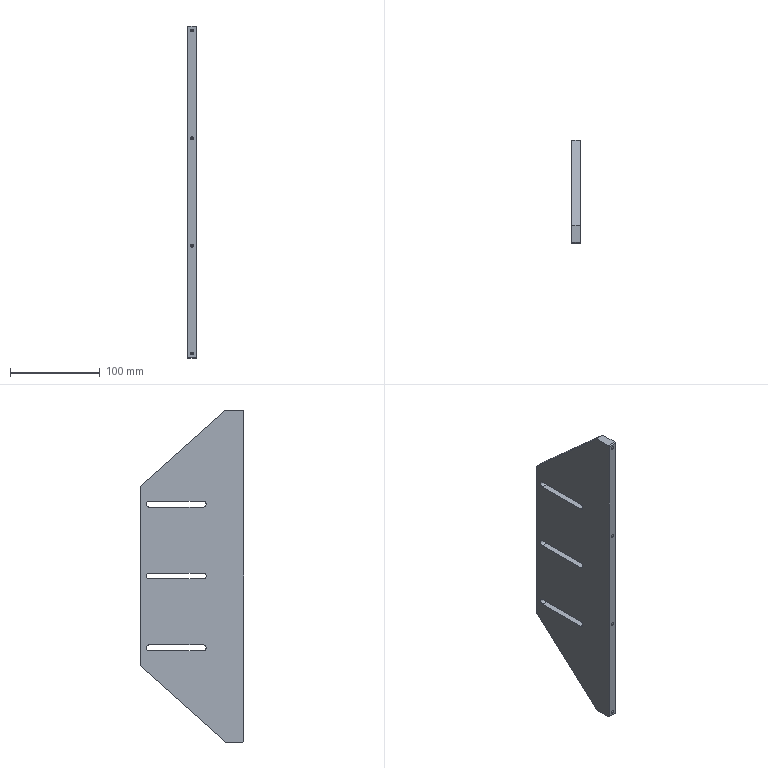Part | SolidWorks | features HoleWzd 2, Chamfer 1, Extrusion 1, ICE 1 | 1 solid | 38 faces | box 10 x 115 x 370 mm | volume 331477 mm3 | plane 16 | cylinder 14 | cone 8 | commonest cylinder face diameters 3.3 x8 6.6 x6
STEP:
#1=CARTESIAN_POINT('',(0.,-104.9,181.65));
#2=VERTEX_POINT('',#1);
#3=CARTESIAN_POINT('',(0.,-104.9,178.35));
#4=VERTEX_POINT('',#3);
#5=CARTESIAN_POINT('',(0.,-104.9,180.));
#6=DIRECTION('',(0.,-1.,0.));
#7=DIRECTION('',(0.,0.,-1.));
#8=AXIS2_PLACEMENT_3D('',#5,#6,#7);
#9=CIRCLE('',#8,1.65);
#10=EDGE_CURVE('',#2,#4,#9,.T.);
#11=ORIENTED_EDGE('',*,*,#10,.F.);
#12=CARTESIAN_POINT('',(0.,-115.,181.65));
#13=VERTEX_POINT('',#12);
#14=CARTESIAN_POINT('',(0.,-115.,181.65));
#15=DIRECTION('',(0.,-1.,0.));
#16=VECTOR('',#15,1000.);
#17=LINE('',#14,#16);
#18=EDGE_CURVE('',#2,#13,#17,.T.);
#19=ORIENTED_EDGE('',*,*,#18,.T.);
#20=CARTESIAN_POINT('',(0.,-115.,178.35));
#21=VERTEX_POINT('',#20);
#22=CARTESIAN_POINT('',(0.,-115.,180.));
#23=DIRECTION('',(0.,-1.,0.));
#24=DIRECTION('',(0.,0.,-1.));
#25=AXIS2_PLACEMENT_3D('',#22,#23,#24);
#26=CIRCLE('',#25,1.65);
#27=EDGE_CURVE('',#13,#21,#26,.T.);
#28=ORIENTED_EDGE('',*,*,#27,.T.);
#29=CARTESIAN_POINT('',(0.,-115.,178.35));
#30=DIRECTION('',(0.,-1.,0.));
#31=VECTOR('',#30,1000.);
#32=LINE('',#29,#31);
#33=EDGE_CURVE('',#4,#21,#32,.T.);
#34=ORIENTED_EDGE('',*,*,#33,.F.);
#35=EDGE_LOOP('',(#11,#19,#28,#34));
#36=FACE_OUTER_BOUND('',#35,.T.);
#37=CARTESIAN_POINT('',(0.,-115.,180.));
#38=DIRECTION('',(0.,-1.,0.));
#39=DIRECTION('',(0.,0.,-1.));
#40=AXIS2_PLACEMENT_3D('',#37,#38,#39);
#41=CYLINDRICAL_SURFACE('',#40,1.65);
#42=ADVANCED_FACE('',(#36),#41,.F.);
#43=CARTESIAN_POINT('',(0.,-103.909,180.));
#44=VERTEX_POINT('',#43);
#45=CARTESIAN_POINT('',(0.,-104.9,178.35));
#46=DIRECTION('',(0.,-0.515,-0.8572));
#47=VECTOR('',#46,1000.);
#48=LINE('',#45,#47);
#49=EDGE_CURVE('',#44,#4,#48,.T.);
#50=ORIENTED_EDGE('',*,*,#49,.F.);
#51=CARTESIAN_POINT('',(0.,-104.9,181.65));
#52=DIRECTION('',(0.,-0.515,0.8572));
#53=VECTOR('',#52,1000.);
#54=LINE('',#51,#53);
#55=EDGE_CURVE('',#44,#2,#54,.T.);
#56=ORIENTED_EDGE('',*,*,#55,.T.);
#57=ORIENTED_EDGE('',*,*,#10,.T.);
#58=EDGE_LOOP('',(#50,#56,#57));
#59=FACE_OUTER_BOUND('',#58,.T.);
#60=CARTESIAN_POINT('',(0.,-104.9,180.));
#61=DIRECTION('',(0.,-1.,0.));
#62=DIRECTION('',(0.,0.,-1.));
#63=AXIS2_PLACEMENT_3D('',#60,#61,#62);
#64=CONICAL_SURFACE('',#63,1.65,1.03);
#65=ADVANCED_FACE('',(#59),#64,.F.);
#66=CARTESIAN_POINT('',(0.,-104.9,61.65));
#67=VERTEX_POINT('',#66);
#68=CARTESIAN_POINT('',(0.,-104.9,58.35));
#69=VERTEX_POINT('',#68);
#70=CARTESIAN_POINT('',(0.,-104.9,60.));
#71=DIRECTION('',(0.,-1.,0.));
#72=DIRECTION('',(0.,0.,-1.));
#73=AXIS2_PLACEMENT_3D('',#70,#71,#72);
#74=CIRCLE('',#73,1.65);
#75=EDGE_CURVE('',#67,#69,#74,.T.);
#76=ORIENTED_EDGE('',*,*,#75,.F.);
#77=CARTESIAN_POINT('',(0.,-115.,61.65));
#78=VERTEX_POINT('',#77);
#79=CARTESIAN_POINT('',(0.,-115.,61.65));
#80=DIRECTION('',(0.,-1.,0.));
#81=VECTOR('',#80,1000.);
#82=LINE('',#79,#81);
#83=EDGE_CURVE('',#67,#78,#82,.T.);
#84=ORIENTED_EDGE('',*,*,#83,.T.);
#85=CARTESIAN_POINT('',(0.,-115.,58.35));
#86=VERTEX_POINT('',#85);
#87=CARTESIAN_POINT('',(0.,-115.,60.));
#88=DIRECTION('',(0.,-1.,0.));
#89=DIRECTION('',(0.,0.,-1.));
#90=AXIS2_PLACEMENT_3D('',#87,#88,#89);
#91=CIRCLE('',#90,1.65);
#92=EDGE_CURVE('',#78,#86,#91,.T.);
#93=ORIENTED_EDGE('',*,*,#92,.T.);
#94=CARTESIAN_POINT('',(0.,-115.,58.35));
#95=DIRECTION('',(0.,-1.,0.));
#96=VECTOR('',#95,1000.);
#97=LINE('',#94,#96);
#98=EDGE_CURVE('',#69,#86,#97,.T.);
#99=ORIENTED_EDGE('',*,*,#98,.F.);
#100=EDGE_LOOP('',(#76,#84,#93,#99));
#101=FACE_OUTER_BOUND('',#100,.T.);
#102=CARTESIAN_POINT('',(0.,-115.,60.));
#103=DIRECTION('',(0.,-1.,0.));
#104=DIRECTION('',(0.,0.,-1.));
#105=AXIS2_PLACEMENT_3D('',#102,#103,#104);
#106=CYLINDRICAL_SURFACE('',#105,1.65);
#107=ADVANCED_FACE('',(#101),#106,.F.);
#108=CARTESIAN_POINT('',(0.,-103.909,60.));
#109=VERTEX_POINT('',#108);
#110=CARTESIAN_POINT('',(0.,-104.9,58.35));
#111=DIRECTION('',(0.,-0.515,-0.8572));
#112=VECTOR('',#111,1000.);
#113=LINE('',#110,#112);
#114=EDGE_CURVE('',#109,#69,#113,.T.);
#115=ORIENTED_EDGE('',*,*,#114,.F.);
#116=CARTESIAN_POINT('',(0.,-104.9,61.65));
#117=DIRECTION('',(0.,-0.515,0.8572));
#118=VECTOR('',#117,1000.);
#119=LINE('',#116,#118);
#120=EDGE_CURVE('',#109,#67,#119,.T.);
#121=ORIENTED_EDGE('',*,*,#120,.T.);
#122=ORIENTED_EDGE('',*,*,#75,.T.);
#123=EDGE_LOOP('',(#115,#121,#122));
#124=FACE_OUTER_BOUND('',#123,.T.);
#125=CARTESIAN_POINT('',(0.,-104.9,60.));
#126=DIRECTION('',(0.,-1.,0.));
#127=DIRECTION('',(0.,0.,-1.));
#128=AXIS2_PLACEMENT_3D('',#125,#126,#127);
#129=CONICAL_SURFACE('',#128,1.65,1.03);
#130=ADVANCED_FACE('',(#124),#129,.F.);
#131=CARTESIAN_POINT('',(0.,-104.9,-58.35));
#132=VERTEX_POINT('',#131);
#133=CARTESIAN_POINT('',(0.,-104.9,-61.65));
#134=VERTEX_POINT('',#133);
#135=CARTESIAN_POINT('',(0.,-104.9,-60.));
#136=DIRECTION('',(0.,-1.,0.));
#137=DIRECTION('',(0.,0.,-1.));
#138=AXIS2_PLACEMENT_3D('',#135,#136,#137);
#139=CIRCLE('',#138,1.65);
#140=EDGE_CURVE('',#132,#134,#139,.T.);
#141=ORIENTED_EDGE('',*,*,#140,.F.);
#142=CARTESIAN_POINT('',(0.,-115.,-58.35));
#143=VERTEX_POINT('',#142);
#144=CARTESIAN_POINT('',(0.,-115.,-58.35));
#145=DIRECTION('',(0.,-1.,0.));
#146=VECTOR('',#145,1000.);
#147=LINE('',#144,#146);
#148=EDGE_CURVE('',#132,#143,#147,.T.);
#149=ORIENTED_EDGE('',*,*,#148,.T.);
#150=CARTESIAN_POINT('',(0.,-115.,-61.65));
#151=VERTEX_POINT('',#150);
#152=CARTESIAN_POINT('',(0.,-115.,-60.));
#153=DIRECTION('',(0.,-1.,0.));
#154=DIRECTION('',(0.,0.,-1.));
#155=AXIS2_PLACEMENT_3D('',#152,#153,#154);
#156=CIRCLE('',#155,1.65);
#157=EDGE_CURVE('',#143,#151,#156,.T.);
#158=ORIENTED_EDGE('',*,*,#157,.T.);
#159=CARTESIAN_POINT('',(0.,-115.,-61.65));
#160=DIRECTION('',(0.,-1.,0.));
#161=VECTOR('',#160,1000.);
#162=LINE('',#159,#161);
#163=EDGE_CURVE('',#134,#151,#162,.T.);
#164=ORIENTED_EDGE('',*,*,#163,.F.);
#165=EDGE_LOOP('',(#141,#149,#158,#164));
#166=FACE_OUTER_BOUND('',#165,.T.);
#167=CARTESIAN_POINT('',(0.,-115.,-60.));
#168=DIRECTION('',(0.,-1.,0.));
#169=DIRECTION('',(0.,0.,-1.));
#170=AXIS2_PLACEMENT_3D('',#167,#168,#169);
#171=CYLINDRICAL_SURFACE('',#170,1.65);
#172=ADVANCED_FACE('',(#166),#171,.F.);
#173=CARTESIAN_POINT('',(0.,-103.909,-60.));
#174=VERTEX_POINT('',#173);
#175=CARTESIAN_POINT('',(0.,-104.9,-61.65));
#176=DIRECTION('',(0.,-0.515,-0.8572));
#177=VECTOR('',#176,1000.);
#178=LINE('',#175,#177);
#179=EDGE_CURVE('',#174,#134,#178,.T.);
#180=ORIENTED_EDGE('',*,*,#179,.F.);
#181=CARTESIAN_POINT('',(0.,-104.9,-58.35));
#182=DIRECTION('',(0.,-0.515,0.8572));
#183=VECTOR('',#182,1000.);
#184=LINE('',#181,#183);
#185=EDGE_CURVE('',#174,#132,#184,.T.);
#186=ORIENTED_EDGE('',*,*,#185,.T.);
#187=ORIENTED_EDGE('',*,*,#140,.T.);
#188=EDGE_LOOP('',(#180,#186,#187));
#189=FACE_OUTER_BOUND('',#188,.T.);
#190=CARTESIAN_POINT('',(0.,-104.9,-60.));
#191=DIRECTION('',(0.,-1.,0.));
#192=DIRECTION('',(0.,0.,-1.));
#193=AXIS2_PLACEMENT_3D('',#190,#191,#192);
#194=CONICAL_SURFACE('',#193,1.65,1.03);
#195=ADVANCED_FACE('',(#189),#194,.F.);
#196=CARTESIAN_POINT('',(0.,-104.9,-178.35));
#197=VERTEX_POINT('',#196);
#198=CARTESIAN_POINT('',(0.,-104.9,-181.65));
#199=VERTEX_POINT('',#198);
#200=CARTESIAN_POINT('',(0.,-104.9,-180.));
#201=DIRECTION('',(0.,-1.,0.));
#202=DIRECTION('',(0.,0.,-1.));
#203=AXIS2_PLACEMENT_3D('',#200,#201,#202);
#204=CIRCLE('',#203,1.65);
#205=EDGE_CURVE('',#197,#199,#204,.T.);
#206=ORIENTED_EDGE('',*,*,#205,.F.);
#207=CARTESIAN_POINT('',(0.,-115.,-178.35));
#208=VERTEX_POINT('',#207);
#209=CARTESIAN_POINT('',(0.,-115.,-178.35));
#210=DIRECTION('',(0.,-1.,0.));
#211=VECTOR('',#210,1000.);
#212=LINE('',#209,#211);
#213=EDGE_CURVE('',#197,#208,#212,.T.);
#214=ORIENTED_EDGE('',*,*,#213,.T.);
#215=CARTESIAN_POINT('',(0.,-115.,-181.65));
#216=VERTEX_POINT('',#215);
#217=CARTESIAN_POINT('',(0.,-115.,-180.));
#218=DIRECTION('',(0.,-1.,0.));
#219=DIRECTION('',(0.,0.,-1.));
#220=AXIS2_PLACEMENT_3D('',#217,#218,#219);
#221=CIRCLE('',#220,1.65);
#222=EDGE_CURVE('',#208,#216,#221,.T.);
#223=ORIENTED_EDGE('',*,*,#222,.T.);
#224=CARTESIAN_POINT('',(0.,-115.,-181.65));
#225=DIRECTION('',(0.,-1.,0.));
#226=VECTOR('',#225,1000.);
#227=LINE('',#224,#226);
#228=EDGE_CURVE('',#199,#216,#227,.T.);
#229=ORIENTED_EDGE('',*,*,#228,.F.);
#230=EDGE_LOOP('',(#206,#214,#223,#229));
#231=FACE_OUTER_BOUND('',#230,.T.);
#232=CARTESIAN_POINT('',(0.,-115.,-180.));
#233=DIRECTION('',(0.,-1.,0.));
#234=DIRECTION('',(0.,0.,-1.));
#235=AXIS2_PLACEMENT_3D('',#232,#233,#234);
#236=CYLINDRICAL_SURFACE('',#235,1.65);
#237=ADVANCED_FACE('',(#231),#236,.F.);
#238=CARTESIAN_POINT('',(0.,-103.909,-180.));
#239=VERTEX_POINT('',#238);
#240=CARTESIAN_POINT('',(0.,-104.9,-181.65));
#241=DIRECTION('',(0.,-0.515,-0.8572));
#242=VECTOR('',#241,1000.);
#243=LINE('',#240,#242);
#244=EDGE_CURVE('',#239,#199,#243,.T.);
#245=ORIENTED_EDGE('',*,*,#244,.F.);
#246=CARTESIAN_POINT('',(0.,-104.9,-178.35));
#247=DIRECTION('',(0.,-0.515,0.8572));
#248=VECTOR('',#247,1000.);
#249=LINE('',#246,#248);
#250=EDGE_CURVE('',#239,#197,#249,.T.);
#251=ORIENTED_EDGE('',*,*,#250,.T.);
#252=ORIENTED_EDGE('',*,*,#205,.T.);
#253=EDGE_LOOP('',(#245,#251,#252));
#254=FACE_OUTER_BOUND('',#253,.T.);
#255=CARTESIAN_POINT('',(0.,-104.9,-180.));
#256=DIRECTION('',(0.,-1.,0.));
#257=DIRECTION('',(0.,0.,-1.));
#258=AXIS2_PLACEMENT_3D('',#255,#256,#257);
#259=CONICAL_SURFACE('',#258,1.65,1.03);
#260=ADVANCED_FACE('',(#254),#259,.F.);
#261=CARTESIAN_POINT('',(-5.,-70.,83.3));
#262=VERTEX_POINT('',#261);
#263=CARTESIAN_POINT('',(-5.,-70.,76.7));
#264=VERTEX_POINT('',#263);
#265=CARTESIAN_POINT('',(-5.,-70.,80.));
#266=DIRECTION('',(1.,0.,0.));
#267=DIRECTION('',(0.,0.,-1.));
#268=AXIS2_PLACEMENT_3D('',#265,#266,#267);
#269=CIRCLE('',#268,3.3);
#270=EDGE_CURVE('',#262,#264,#269,.T.);
#271=ORIENTED_EDGE('',*,*,#270,.T.);
#272=CARTESIAN_POINT('',(-5.,-10.,76.7));
#273=VERTEX_POINT('',#272);
#274=CARTESIAN_POINT('',(-5.,-70.,76.7));
#275=DIRECTION('',(0.,1.,0.));
#276=VECTOR('',#275,1000.);
#277=LINE('',#274,#276);
#278=EDGE_CURVE('',#264,#273,#277,.T.);
#279=ORIENTED_EDGE('',*,*,#278,.T.);
#280=CARTESIAN_POINT('',(-5.,-10.,83.3));
#281=VERTEX_POINT('',#280);
#282=CARTESIAN_POINT('',(-5.,-10.,80.));
#283=DIRECTION('',(1.,0.,0.));
#284=DIRECTION('',(0.,0.,-1.));
#285=AXIS2_PLACEMENT_3D('',#282,#283,#284);
#286=CIRCLE('',#285,3.3);
#287=EDGE_CURVE('',#273,#281,#286,.T.);
#288=ORIENTED_EDGE('',*,*,#287,.T.);
#289=CARTESIAN_POINT('',(-5.,-70.,83.3));
#290=DIRECTION('',(0.,1.,0.));
#291=VECTOR('',#290,1000.);
#292=LINE('',#289,#291);
#293=EDGE_CURVE('',#262,#281,#292,.T.);
#294=ORIENTED_EDGE('',*,*,#293,.F.);
#295=EDGE_LOOP('',(#271,#279,#288,#294));
#296=FACE_BOUND('',#295,.T.);
#297=CARTESIAN_POINT('',(-5.,-70.,3.3));
#298=VERTEX_POINT('',#297);
#299=CARTESIAN_POINT('',(-5.,-10.,3.3));
#300=VERTEX_POINT('',#299);
#301=CARTESIAN_POINT('',(-5.,-70.,3.3));
#302=DIRECTION('',(0.,1.,0.));
#303=VECTOR('',#302,1000.);
#304=LINE('',#301,#303);
#305=EDGE_CURVE('',#298,#300,#304,.T.);
#306=ORIENTED_EDGE('',*,*,#305,.F.);
#307=CARTESIAN_POINT('',(-5.,-70.,-3.3));
#308=VERTEX_POINT('',#307);
#309=CARTESIAN_POINT('',(-5.,-70.,0.));
#310=DIRECTION('',(1.,0.,0.));
#311=DIRECTION('',(0.,0.,-1.));
#312=AXIS2_PLACEMENT_3D('',#309,#310,#311);
#313=CIRCLE('',#312,3.3);
#314=EDGE_CURVE('',#298,#308,#313,.T.);
#315=ORIENTED_EDGE('',*,*,#314,.T.);
#316=CARTESIAN_POINT('',(-5.,-10.,-3.3));
#317=VERTEX_POINT('',#316);
#318=CARTESIAN_POINT('',(-5.,-70.,-3.3));
#319=DIRECTION('',(0.,1.,0.));
#320=VECTOR('',#319,1000.);
#321=LINE('',#318,#320);
#322=EDGE_CURVE('',#308,#317,#321,.T.);
#323=ORIENTED_EDGE('',*,*,#322,.T.);
#324=CARTESIAN_POINT('',(-5.,-10.,0.));
#325=DIRECTION('',(1.,0.,0.));
#326=DIRECTION('',(0.,0.,-1.));
#327=AXIS2_PLACEMENT_3D('',#324,#325,#326);
#328=CIRCLE('',#327,3.3);
#329=EDGE_CURVE('',#317,#300,#328,.T.);
#330=ORIENTED_EDGE('',*,*,#329,.T.);
#331=EDGE_LOOP('',(#306,#315,#323,#330));
#332=FACE_BOUND('',#331,.T.);
#333=CARTESIAN_POINT('',(-5.,-114.,-185.));
#334=VERTEX_POINT('',#333);
#335=CARTESIAN_POINT('',(-5.,-95.,-185.));
#336=VERTEX_POINT('',#335);
#337=CARTESIAN_POINT('',(-5.,-95.,-185.));
#338=DIRECTION('',(0.,1.,0.));
#339=VECTOR('',#338,1000.);
#340=LINE('',#337,#339);
#341=EDGE_CURVE('',#334,#336,#340,.T.);
#342=ORIENTED_EDGE('',*,*,#341,.F.);
#343=CARTESIAN_POINT('',(-5.,-115.,-184.));
#344=VERTEX_POINT('',#343);
#345=CARTESIAN_POINT('',(-5.,-149.5,-149.5));
#346=DIRECTION('',(0.,-0.7071,0.7071));
#347=VECTOR('',#346,1000.);
#348=LINE('',#345,#347);
#349=EDGE_CURVE('',#334,#344,#348,.T.);
#350=ORIENTED_EDGE('',*,*,#349,.T.);
#351=CARTESIAN_POINT('',(-5.,-115.,184.));
#352=VERTEX_POINT('',#351);
#353=CARTESIAN_POINT('',(-5.,-115.,-185.));
#354=DIRECTION('',(0.,0.,-1.));
#355=VECTOR('',#354,1000.);
#356=LINE('',#353,#355);
#357=EDGE_CURVE('',#352,#344,#356,.T.);
#358=ORIENTED_EDGE('',*,*,#357,.F.);
#359=CARTESIAN_POINT('',(-5.,-114.,185.));
#360=VERTEX_POINT('',#359);
#361=CARTESIAN_POINT('',(-5.,-149.5,149.5));
#362=DIRECTION('',(0.,0.7071,0.7071));
#363=VECTOR('',#362,1000.);
#364=LINE('',#361,#363);
#365=EDGE_CURVE('',#352,#360,#364,.T.);
#366=ORIENTED_EDGE('',*,*,#365,.T.);
#367=CARTESIAN_POINT('',(-5.,-95.,185.));
#368=VERTEX_POINT('',#367);
#369=CARTESIAN_POINT('',(-5.,-95.,185.));
#370=DIRECTION('',(0.,-1.,0.));
#371=VECTOR('',#370,1000.);
#372=LINE('',#369,#371);
#373=EDGE_CURVE('',#368,#360,#372,.T.);
#374=ORIENTED_EDGE('',*,*,#373,.F.);
#375=CARTESIAN_POINT('',(-5.,0.,100.));
#376=VERTEX_POINT('',#375);
#377=CARTESIAN_POINT('',(-5.,0.,100.));
#378=DIRECTION('',(0.,-0.7452,0.6668));
#379=VECTOR('',#378,1000.);
#380=LINE('',#377,#379);
#381=EDGE_CURVE('',#376,#368,#380,.T.);
#382=ORIENTED_EDGE('',*,*,#381,.F.);
#383=CARTESIAN_POINT('',(-5.,0.,-100.));
#384=VERTEX_POINT('',#383);
#385=CARTESIAN_POINT('',(-5.,0.,100.));
#386=DIRECTION('',(0.,0.,1.));
#387=VECTOR('',#386,1000.);
#388=LINE('',#385,#387);
#389=EDGE_CURVE('',#384,#376,#388,.T.);
#390=ORIENTED_EDGE('',*,*,#389,.F.);
#391=CARTESIAN_POINT('',(-5.,0.,-100.));
#392=DIRECTION('',(0.,0.7452,0.6668));
#393=VECTOR('',#392,1000.);
#394=LINE('',#391,#393);
#395=EDGE_CURVE('',#336,#384,#394,.T.);
#396=ORIENTED_EDGE('',*,*,#395,.F.);
#397=EDGE_LOOP('',(#342,#350,#358,#366,#374,#382,#390,#396));
#398=FACE_OUTER_BOUND('',#397,.T.);
#399=CARTESIAN_POINT('',(-5.,-70.,-83.3));
#400=VERTEX_POINT('',#399);
#401=CARTESIAN_POINT('',(-5.,-10.,-83.3));
#402=VERTEX_POINT('',#401);
#403=CARTESIAN_POINT('',(-5.,-70.,-83.3));
#404=DIRECTION('',(0.,1.,0.));
#405=VECTOR('',#404,1000.);
#406=LINE('',#403,#405);
#407=EDGE_CURVE('',#400,#402,#406,.T.);
#408=ORIENTED_EDGE('',*,*,#407,.T.);
#409=CARTESIAN_POINT('',(-5.,-10.,-76.7));
#410=VERTEX_POINT('',#409);
#411=CARTESIAN_POINT('',(-5.,-10.,-80.));
#412=DIRECTION('',(1.,0.,0.));
#413=DIRECTION('',(0.,0.,-1.));
#414=AXIS2_PLACEMENT_3D('',#411,#412,#413);
#415=CIRCLE('',#414,3.3);
#416=EDGE_CURVE('',#402,#410,#415,.T.);
#417=ORIENTED_EDGE('',*,*,#416,.T.);
#418=CARTESIAN_POINT('',(-5.,-70.,-76.7));
#419=VERTEX_POINT('',#418);
#420=CARTESIAN_POINT('',(-5.,-70.,-76.7));
#421=DIRECTION('',(0.,1.,0.));
#422=VECTOR('',#421,1000.);
#423=LINE('',#420,#422);
#424=EDGE_CURVE('',#419,#410,#423,.T.);
#425=ORIENTED_EDGE('',*,*,#424,.F.);
#426=CARTESIAN_POINT('',(-5.,-70.,-80.));
#427=DIRECTION('',(1.,0.,0.));
#428=DIRECTION('',(0.,0.,-1.));
#429=AXIS2_PLACEMENT_3D('',#426,#427,#428);
#430=CIRCLE('',#429,3.3);
#431=EDGE_CURVE('',#419,#400,#430,.T.);
#432=ORIENTED_EDGE('',*,*,#431,.T.);
#433=EDGE_LOOP('',(#408,#417,#425,#432));
#434=FACE_BOUND('',#433,.T.);
#435=CARTESIAN_POINT('',(-5.,0.,0.));
#436=DIRECTION('',(-1.,0.,0.));
#437=DIRECTION('',(0.,0.,1.));
#438=AXIS2_PLACEMENT_3D('',#435,#436,#437);
#439=PLANE('',#438);
#440=ADVANCED_FACE('',(#296,#332,#398,#434),#439,.T.);
#441=ORIENTED_EDGE('',*,*,#395,.T.);
#442=CARTESIAN_POINT('',(5.,0.,-100.));
#443=VERTEX_POINT('',#442);
#444=CARTESIAN_POINT('',(5.,0.,-100.));
#445=DIRECTION('',(-1.,0.,0.));
#446=VECTOR('',#445,1000.);
#447=LINE('',#444,#446);
#448=EDGE_CURVE('',#443,#384,#447,.T.);
#449=ORIENTED_EDGE('',*,*,#448,.F.);
#450=CARTESIAN_POINT('',(5.,-95.,-185.));
#451=VERTEX_POINT('',#450);
#452=CARTESIAN_POINT('',(5.,0.,-100.));
#453=DIRECTION('',(0.,0.7452,0.6668));
#454=VECTOR('',#453,1000.);
#455=LINE('',#452,#454);
#456=EDGE_CURVE('',#451,#443,#455,.T.);
#457=ORIENTED_EDGE('',*,*,#456,.F.);
#458=CARTESIAN_POINT('',(5.,-95.,-185.));
#459=DIRECTION('',(-1.,0.,0.));
#460=VECTOR('',#459,1000.);
#461=LINE('',#458,#460);
#462=EDGE_CURVE('',#451,#336,#461,.T.);
#463=ORIENTED_EDGE('',*,*,#462,.T.);
#464=EDGE_LOOP('',(#441,#449,#457,#463));
#465=FACE_OUTER_BOUND('',#464,.T.);
#466=CARTESIAN_POINT('',(5.,0.,-100.));
#467=DIRECTION('',(0.,-0.6668,0.7452));
#468=DIRECTION('',(0.,-0.7452,-0.6668));
#469=AXIS2_PLACEMENT_3D('',#466,#467,#468);
#470=PLANE('',#469);
#471=ADVANCED_FACE('',(#465),#470,.F.);
#472=ORIENTED_EDGE('',*,*,#389,.T.);
#473=CARTESIAN_POINT('',(5.,0.,100.));
#474=VERTEX_POINT('',#473);
#475=CARTESIAN_POINT('',(5.,0.,100.));
#476=DIRECTION('',(-1.,0.,0.));
#477=VECTOR('',#476,1000.);
#478=LINE('',#475,#477);
#479=EDGE_CURVE('',#474,#376,#478,.T.);
#480=ORIENTED_EDGE('',*,*,#479,.F.);
#481=CARTESIAN_POINT('',(5.,0.,100.));
#482=DIRECTION('',(0.,0.,1.));
#483=VECTOR('',#482,1000.);
#484=LINE('',#481,#483);
#485=EDGE_CURVE('',#443,#474,#484,.T.);
#486=ORIENTED_EDGE('',*,*,#485,.F.);
#487=ORIENTED_EDGE('',*,*,#448,.T.);
#488=EDGE_LOOP('',(#472,#480,#486,#487));
#489=FACE_OUTER_BOUND('',#488,.T.);
#490=CARTESIAN_POINT('',(5.,0.,100.));
#491=DIRECTION('',(0.,-1.,0.));
#492=DIRECTION('',(0.,0.,-1.));
#493=AXIS2_PLACEMENT_3D('',#490,#491,#492);
#494=PLANE('',#493);
#495=ADVANCED_FACE('',(#489),#494,.F.);
#496=ORIENTED_EDGE('',*,*,#381,.T.);
#497=CARTESIAN_POINT('',(5.,-95.,185.));
#498=VERTEX_POINT('',#497);
#499=CARTESIAN_POINT('',(5.,-95.,185.));
#500=DIRECTION('',(-1.,0.,0.));
#501=VECTOR('',#500,1000.);
#502=LINE('',#499,#501);
#503=EDGE_CURVE('',#498,#368,#502,.T.);
#504=ORIENTED_EDGE('',*,*,#503,.F.);
#505=CARTESIAN_POINT('',(5.,0.,100.));
#506=DIRECTION('',(0.,-0.7452,0.6668));
#507=VECTOR('',#506,1000.);
#508=LINE('',#505,#507);
#509=EDGE_CURVE('',#474,#498,#508,.T.);
#510=ORIENTED_EDGE('',*,*,#509,.F.);
#511=ORIENTED_EDGE('',*,*,#479,.T.);
#512=EDGE_LOOP('',(#496,#504,#510,#511));
#513=FACE_OUTER_BOUND('',#512,.T.);
#514=CARTESIAN_POINT('',(5.,0.,100.));
#515=DIRECTION('',(0.,-0.6668,-0.7452));
#516=DIRECTION('',(0.,0.7452,-0.6668));
#517=AXIS2_PLACEMENT_3D('',#514,#515,#516);
#518=PLANE('',#517);
#519=ADVANCED_FACE('',(#513),#518,.F.);
#520=ORIENTED_EDGE('',*,*,#373,.T.);
#521=CARTESIAN_POINT('',(5.,-114.,185.));
#522=VERTEX_POINT('',#521);
#523=CARTESIAN_POINT('',(5.,-114.,185.));
#524=DIRECTION('',(1.,0.,0.));
#525=VECTOR('',#524,1000.);
#526=LINE('',#523,#525);
#527=EDGE_CURVE('',#360,#522,#526,.T.);
#528=ORIENTED_EDGE('',*,*,#527,.T.);
#529=CARTESIAN_POINT('',(5.,-95.,185.));
#530=DIRECTION('',(0.,-1.,0.));
#531=VECTOR('',#530,1000.);
#532=LINE('',#529,#531);
#533=EDGE_CURVE('',#498,#522,#532,.T.);
#534=ORIENTED_EDGE('',*,*,#533,.F.);
#535=ORIENTED_EDGE('',*,*,#503,.T.);
#536=EDGE_LOOP('',(#520,#528,#534,#535));
#537=FACE_OUTER_BOUND('',#536,.T.);
#538=CARTESIAN_POINT('',(5.,-95.,185.));
#539=DIRECTION('',(0.,0.,-1.));
#540=DIRECTION('',(0.,1.,0.));
#541=AXIS2_PLACEMENT_3D('',#538,#539,#540);
#542=PLANE('',#541);
#543=ADVANCED_FACE('',(#537),#542,.F.);
#544=CARTESIAN_POINT('',(0.,-115.,180.));
#545=DIRECTION('',(0.,-1.,0.));
#546=DIRECTION('',(0.,0.,-1.));
#547=AXIS2_PLACEMENT_3D('',#544,#545,#546);
#548=CIRCLE('',#547,1.65);
#549=EDGE_CURVE('',#21,#13,#548,.T.);
#550=ORIENTED_EDGE('',*,*,#549,.F.);
#551=ORIENTED_EDGE('',*,*,#27,.F.);
#552=EDGE_LOOP('',(#550,#551));
#553=FACE_BOUND('',#552,.T.);
#554=CARTESIAN_POINT('',(0.,-115.,60.));
#555=DIRECTION('',(0.,-1.,0.));
#556=DIRECTION('',(0.,0.,-1.));
#557=AXIS2_PLACEMENT_3D('',#554,#555,#556);
#558=CIRCLE('',#557,1.65);
#559=EDGE_CURVE('',#86,#78,#558,.T.);
#560=ORIENTED_EDGE('',*,*,#559,.F.);
#561=ORIENTED_EDGE('',*,*,#92,.F.);
#562=EDGE_LOOP('',(#560,#561));
#563=FACE_BOUND('',#562,.T.);
#564=CARTESIAN_POINT('',(0.,-115.,-60.));
#565=DIRECTION('',(0.,-1.,0.));
#566=DIRECTION('',(0.,0.,-1.));
#567=AXIS2_PLACEMENT_3D('',#564,#565,#566);
#568=CIRCLE('',#567,1.65);
#569=EDGE_CURVE('',#151,#143,#568,.T.);
#570=ORIENTED_EDGE('',*,*,#569,.F.);
#571=ORIENTED_EDGE('',*,*,#157,.F.);
#572=EDGE_LOOP('',(#570,#571));
#573=FACE_BOUND('',#572,.T.);
#574=CARTESIAN_POINT('',(0.,-115.,-180.));
#575=DIRECTION('',(0.,-1.,0.));
#576=DIRECTION('',(0.,0.,-1.));
#577=AXIS2_PLACEMENT_3D('',#574,#575,#576);
#578=CIRCLE('',#577,1.65);
#579=EDGE_CURVE('',#216,#208,#578,.T.);
#580=ORIENTED_EDGE('',*,*,#579,.F.);
#581=ORIENTED_EDGE('',*,*,#222,.F.);
#582=EDGE_LOOP('',(#580,#581));
#583=FACE_BOUND('',#582,.T.);
#584=ORIENTED_EDGE('',*,*,#357,.T.);
#585=CARTESIAN_POINT('',(5.,-115.,-184.));
#586=VERTEX_POINT('',#585);
#587=CARTESIAN_POINT('',(5.,-115.,-184.));
#588=DIRECTION('',(1.,0.,0.));
#589=VECTOR('',#588,1000.);
#590=LINE('',#587,#589);
#591=EDGE_CURVE('',#344,#586,#590,.T.);
#592=ORIENTED_EDGE('',*,*,#591,.T.);
#593=CARTESIAN_POINT('',(5.,-115.,184.));
#594=VERTEX_POINT('',#593);
#595=CARTESIAN_POINT('',(5.,-115.,-185.));
#596=DIRECTION('',(0.,0.,-1.));
#597=VECTOR('',#596,1000.);
#598=LINE('',#595,#597);
#599=EDGE_CURVE('',#594,#586,#598,.T.);
#600=ORIENTED_EDGE('',*,*,#599,.F.);
#601=CARTESIAN_POINT('',(5.,-115.,184.));
#602=DIRECTION('',(-1.,0.,0.));
#603=VECTOR('',#602,1000.);
#604=LINE('',#601,#603);
#605=EDGE_CURVE('',#594,#352,#604,.T.);
#606=ORIENTED_EDGE('',*,*,#605,.T.);
#607=EDGE_LOOP('',(#584,#592,#600,#606));
#608=FACE_OUTER_BOUND('',#607,.T.);
#609=CARTESIAN_POINT('',(5.,-115.,-185.));
#610=DIRECTION('',(0.,1.,0.));
#611=DIRECTION('',(0.,0.,1.));
#612=AXIS2_PLACEMENT_3D('',#609,#610,#611);
#613=PLANE('',#612);
#614=ADVANCED_FACE('',(#553,#563,#573,#583,#608),#613,.F.);
#615=CARTESIAN_POINT('',(5.,-114.,-185.));
#616=VERTEX_POINT('',#615);
#617=CARTESIAN_POINT('',(5.,-95.,-185.));
#618=DIRECTION('',(0.,1.,0.));
#619=VECTOR('',#618,1000.);
#620=LINE('',#617,#619);
#621=EDGE_CURVE('',#616,#451,#620,.T.);
#622=ORIENTED_EDGE('',*,*,#621,.F.);
#623=CARTESIAN_POINT('',(5.,-114.,-185.));
#624=DIRECTION('',(-1.,0.,0.));
#625=VECTOR('',#624,1000.);
#626=LINE('',#623,#625);
#627=EDGE_CURVE('',#616,#334,#626,.T.);
#628=ORIENTED_EDGE('',*,*,#627,.T.);
#629=ORIENTED_EDGE('',*,*,#341,.T.);
#630=ORIENTED_EDGE('',*,*,#462,.F.);
#631=EDGE_LOOP('',(#622,#628,#629,#630));
#632=FACE_OUTER_BOUND('',#631,.T.);
#633=CARTESIAN_POINT('',(5.,-95.,-185.));
#634=DIRECTION('',(0.,0.,1.));
#635=DIRECTION('',(0.,-1.,0.));
#636=AXIS2_PLACEMENT_3D('',#633,#634,#635);
#637=PLANE('',#636);
#638=ADVANCED_FACE('',(#632),#637,.F.);
#639=CARTESIAN_POINT('',(5.,-70.,83.3));
#640=VERTEX_POINT('',#639);
#641=CARTESIAN_POINT('',(5.,-70.,76.7));
#642=VERTEX_POINT('',#641);
#643=CARTESIAN_POINT('',(5.,-70.,80.));
#644=DIRECTION('',(1.,0.,0.));
#645=DIRECTION('',(0.,0.,-1.));
#646=AXIS2_PLACEMENT_3D('',#643,#644,#645);
#647=CIRCLE('',#646,3.3);
#648=EDGE_CURVE('',#640,#642,#647,.T.);
#649=ORIENTED_EDGE('',*,*,#648,.F.);
#650=CARTESIAN_POINT('',(5.,-10.,83.3));
#651=VERTEX_POINT('',#650);
#652=CARTESIAN_POINT('',(5.,-70.,83.3));
#653=DIRECTION('',(0.,1.,0.));
#654=VECTOR('',#653,1000.);
#655=LINE('',#652,#654);
#656=EDGE_CURVE('',#640,#651,#655,.T.);
#657=ORIENTED_EDGE('',*,*,#656,.T.);
#658=CARTESIAN_POINT('',(5.,-10.,76.7));
#659=VERTEX_POINT('',#658);
#660=CARTESIAN_POINT('',(5.,-10.,80.));
#661=DIRECTION('',(1.,0.,0.));
#662=DIRECTION('',(0.,0.,-1.));
#663=AXIS2_PLACEMENT_3D('',#660,#661,#662);
#664=CIRCLE('',#663,3.3);
#665=EDGE_CURVE('',#659,#651,#664,.T.);
#666=ORIENTED_EDGE('',*,*,#665,.F.);
#667=CARTESIAN_POINT('',(5.,-70.,76.7));
#668=DIRECTION('',(0.,1.,0.));
#669=VECTOR('',#668,1000.);
#670=LINE('',#667,#669);
#671=EDGE_CURVE('',#642,#659,#670,.T.);
#672=ORIENTED_EDGE('',*,*,#671,.F.);
#673=EDGE_LOOP('',(#649,#657,#666,#672));
#674=FACE_BOUND('',#673,.T.);
#675=CARTESIAN_POINT('',(5.,-70.,3.3));
#676=VERTEX_POINT('',#675);
#677=CARTESIAN_POINT('',(5.,-70.,-3.3));
#678=VERTEX_POINT('',#677);
#679=CARTESIAN_POINT('',(5.,-70.,0.));
#680=DIRECTION('',(1.,0.,0.));
#681=DIRECTION('',(0.,0.,-1.));
#682=AXIS2_PLACEMENT_3D('',#679,#680,#681);
#683=CIRCLE('',#682,3.3);
#684=EDGE_CURVE('',#676,#678,#683,.T.);
#685=ORIENTED_EDGE('',*,*,#684,.F.);
#686=CARTESIAN_POINT('',(5.,-10.,3.3));
#687=VERTEX_POINT('',#686);
#688=CARTESIAN_POINT('',(5.,-70.,3.3));
#689=DIRECTION('',(0.,1.,0.));
#690=VECTOR('',#689,1000.);
#691=LINE('',#688,#690);
#692=EDGE_CURVE('',#676,#687,#691,.T.);
#693=ORIENTED_EDGE('',*,*,#692,.T.);
#694=CARTESIAN_POINT('',(5.,-10.,-3.3));
#695=VERTEX_POINT('',#694);
#696=CARTESIAN_POINT('',(5.,-10.,0.));
#697=DIRECTION('',(1.,0.,0.));
#698=DIRECTION('',(0.,0.,-1.));
#699=AXIS2_PLACEMENT_3D('',#696,#697,#698);
#700=CIRCLE('',#699,3.3);
#701=EDGE_CURVE('',#695,#687,#700,.T.);
#702=ORIENTED_EDGE('',*,*,#701,.F.);
#703=CARTESIAN_POINT('',(5.,-70.,-3.3));
#704=DIRECTION('',(0.,1.,0.));
#705=VECTOR('',#704,1000.);
#706=LINE('',#703,#705);
#707=EDGE_CURVE('',#678,#695,#706,.T.);
#708=ORIENTED_EDGE('',*,*,#707,.F.);
#709=EDGE_LOOP('',(#685,#693,#702,#708));
#710=FACE_BOUND('',#709,.T.);
#711=CARTESIAN_POINT('',(5.,-70.,-76.7));
#712=VERTEX_POINT('',#711);
#713=CARTESIAN_POINT('',(5.,-70.,-83.3));
#714=VERTEX_POINT('',#713);
#715=CARTESIAN_POINT('',(5.,-70.,-80.));
#716=DIRECTION('',(1.,0.,0.));
#717=DIRECTION('',(0.,0.,-1.));
#718=AXIS2_PLACEMENT_3D('',#715,#716,#717);
#719=CIRCLE('',#718,3.3);
#720=EDGE_CURVE('',#712,#714,#719,.T.);
#721=ORIENTED_EDGE('',*,*,#720,.F.);
#722=CARTESIAN_POINT('',(5.,-10.,-76.7));
#723=VERTEX_POINT('',#722);
#724=CARTESIAN_POINT('',(5.,-70.,-76.7));
#725=DIRECTION('',(0.,1.,0.));
#726=VECTOR('',#725,1000.);
#727=LINE('',#724,#726);
#728=EDGE_CURVE('',#712,#723,#727,.T.);
#729=ORIENTED_EDGE('',*,*,#728,.T.);
#730=CARTESIAN_POINT('',(5.,-10.,-83.3));
#731=VERTEX_POINT('',#730);
#732=CARTESIAN_POINT('',(5.,-10.,-80.));
#733=DIRECTION('',(1.,0.,0.));
#734=DIRECTION('',(0.,0.,-1.));
#735=AXIS2_PLACEMENT_3D('',#732,#733,#734);
#736=CIRCLE('',#735,3.3);
#737=EDGE_CURVE('',#731,#723,#736,.T.);
#738=ORIENTED_EDGE('',*,*,#737,.F.);
#739=CARTESIAN_POINT('',(5.,-70.,-83.3));
#740=DIRECTION('',(0.,1.,0.));
#741=VECTOR('',#740,1000.);
#742=LINE('',#739,#741);
#743=EDGE_CURVE('',#714,#731,#742,.T.);
#744=ORIENTED_EDGE('',*,*,#743,.F.);
#745=EDGE_LOOP('',(#721,#729,#738,#744));
#746=FACE_BOUND('',#745,.T.);
#747=ORIENTED_EDGE('',*,*,#599,.T.);
#748=CARTESIAN_POINT('',(5.,-114.,-185.));
#749=DIRECTION('',(0.,0.7071,-0.7071));
#750=VECTOR('',#749,1000.);
#751=LINE('',#748,#750);
#752=EDGE_CURVE('',#586,#616,#751,.T.);
#753=ORIENTED_EDGE('',*,*,#752,.T.);
#754=ORIENTED_EDGE('',*,*,#621,.T.);
#755=ORIENTED_EDGE('',*,*,#456,.T.);
#756=ORIENTED_EDGE('',*,*,#485,.T.);
#757=ORIENTED_EDGE('',*,*,#509,.T.);
#758=ORIENTED_EDGE('',*,*,#533,.T.);
#759=CARTESIAN_POINT('',(5.,-115.,184.));
#760=DIRECTION('',(0.,-0.7071,-0.7071));
#761=VECTOR('',#760,1000.);
#762=LINE('',#759,#761);
#763=EDGE_CURVE('',#522,#594,#762,.T.);
#764=ORIENTED_EDGE('',*,*,#763,.T.);
#765=EDGE_LOOP('',(#747,#753,#754,#755,#756,#757,#758,#764));
#766=FACE_OUTER_BOUND('',#765,.T.);
#767=CARTESIAN_POINT('',(5.,0.,0.));
#768=DIRECTION('',(-1.,0.,0.));
#769=DIRECTION('',(0.,0.,1.));
#770=AXIS2_PLACEMENT_3D('',#767,#768,#769);
#771=PLANE('',#770);
#772=ADVANCED_FACE('',(#674,#710,#746,#766),#771,.F.);
#773=ORIENTED_EDGE('',*,*,#752,.F.);
#774=ORIENTED_EDGE('',*,*,#591,.F.);
#775=ORIENTED_EDGE('',*,*,#349,.F.);
#776=ORIENTED_EDGE('',*,*,#627,.F.);
#777=EDGE_LOOP('',(#773,#774,#775,#776));
#778=FACE_OUTER_BOUND('',#777,.T.);
#779=CARTESIAN_POINT('',(5.,-114.,-185.));
#780=DIRECTION('',(0.,0.7071,0.7071));
#781=DIRECTION('',(-1.,0.,0.));
#782=AXIS2_PLACEMENT_3D('',#779,#780,#781);
#783=PLANE('',#782);
#784=ADVANCED_FACE('',(#778),#783,.F.);
#785=ORIENTED_EDGE('',*,*,#763,.F.);
#786=ORIENTED_EDGE('',*,*,#527,.F.);
#787=ORIENTED_EDGE('',*,*,#365,.F.);
#788=ORIENTED_EDGE('',*,*,#605,.F.);
#789=EDGE_LOOP('',(#785,#786,#787,#788));
#790=FACE_OUTER_BOUND('',#789,.T.);
#791=CARTESIAN_POINT('',(5.,-115.,184.));
#792=DIRECTION('',(0.,0.7071,-0.7071));
#793=DIRECTION('',(-1.,0.,0.));
#794=AXIS2_PLACEMENT_3D('',#791,#792,#793);
#795=PLANE('',#794);
#796=ADVANCED_FACE('',(#790),#795,.F.);
#797=ORIENTED_EDGE('',*,*,#416,.F.);
#798=CARTESIAN_POINT('',(5.,-10.,-83.3));
#799=DIRECTION('',(-1.,0.,0.));
#800=VECTOR('',#799,1000.);
#801=LINE('',#798,#800);
#802=EDGE_CURVE('',#731,#402,#801,.T.);
#803=ORIENTED_EDGE('',*,*,#802,.F.);
#804=ORIENTED_EDGE('',*,*,#737,.T.);
#805=CARTESIAN_POINT('',(5.,-10.,-76.7));
#806=DIRECTION('',(1.,0.,0.));
#807=VECTOR('',#806,1000.);
#808=LINE('',#805,#807);
#809=EDGE_CURVE('',#410,#723,#808,.T.);
#810=ORIENTED_EDGE('',*,*,#809,.F.);
#811=EDGE_LOOP('',(#797,#803,#804,#810));
#812=FACE_OUTER_BOUND('',#811,.T.);
#813=CARTESIAN_POINT('',(5.,-10.,-80.));
#814=DIRECTION('',(1.,0.,0.));
#815=DIRECTION('',(0.,0.,-1.));
#816=AXIS2_PLACEMENT_3D('',#813,#814,#815);
#817=CYLINDRICAL_SURFACE('',#816,3.3);
#818=ADVANCED_FACE('',(#812),#817,.F.);
#819=ORIENTED_EDGE('',*,*,#720,.T.);
#820=CARTESIAN_POINT('',(5.,-70.,-83.3));
#821=DIRECTION('',(1.,0.,0.));
#822=VECTOR('',#821,1000.);
#823=LINE('',#820,#822);
#824=EDGE_CURVE('',#400,#714,#823,.T.);
#825=ORIENTED_EDGE('',*,*,#824,.F.);
#826=ORIENTED_EDGE('',*,*,#431,.F.);
#827=CARTESIAN_POINT('',(5.,-70.,-76.7));
#828=DIRECTION('',(-1.,0.,0.));
#829=VECTOR('',#828,1000.);
#830=LINE('',#827,#829);
#831=EDGE_CURVE('',#712,#419,#830,.T.);
#832=ORIENTED_EDGE('',*,*,#831,.F.);
#833=EDGE_LOOP('',(#819,#825,#826,#832));
#834=FACE_OUTER_BOUND('',#833,.T.);
#835=CARTESIAN_POINT('',(5.,-70.,-80.));
#836=DIRECTION('',(1.,0.,0.));
#837=DIRECTION('',(0.,0.,-1.));
#838=AXIS2_PLACEMENT_3D('',#835,#836,#837);
#839=CYLINDRICAL_SURFACE('',#838,3.3);
#840=ADVANCED_FACE('',(#834),#839,.F.);
#841=ORIENTED_EDGE('',*,*,#809,.T.);
#842=ORIENTED_EDGE('',*,*,#728,.F.);
#843=ORIENTED_EDGE('',*,*,#831,.T.);
#844=ORIENTED_EDGE('',*,*,#424,.T.);
#845=EDGE_LOOP('',(#841,#842,#843,#844));
#846=FACE_OUTER_BOUND('',#845,.T.);
#847=CARTESIAN_POINT('',(5.,-70.,-76.7));
#848=DIRECTION('',(0.,0.,1.));
#849=DIRECTION('',(1.,0.,0.));
#850=AXIS2_PLACEMENT_3D('',#847,#848,#849);
#851=PLANE('',#850);
#852=ADVANCED_FACE('',(#846),#851,.F.);
#853=ORIENTED_EDGE('',*,*,#802,.T.);
#854=ORIENTED_EDGE('',*,*,#407,.F.);
#855=ORIENTED_EDGE('',*,*,#824,.T.);
#856=ORIENTED_EDGE('',*,*,#743,.T.);
#857=EDGE_LOOP('',(#853,#854,#855,#856));
#858=FACE_OUTER_BOUND('',#857,.T.);
#859=CARTESIAN_POINT('',(5.,-70.,-83.3));
#860=DIRECTION('',(0.,0.,-1.));
#861=DIRECTION('',(-1.,0.,0.));
#862=AXIS2_PLACEMENT_3D('',#859,#860,#861);
#863=PLANE('',#862);
#864=ADVANCED_FACE('',(#858),#863,.F.);
#865=ORIENTED_EDGE('',*,*,#329,.F.);
#866=CARTESIAN_POINT('',(5.,-10.,-3.3));
#867=DIRECTION('',(-1.,0.,0.));
#868=VECTOR('',#867,1000.);
#869=LINE('',#866,#868);
#870=EDGE_CURVE('',#695,#317,#869,.T.);
#871=ORIENTED_EDGE('',*,*,#870,.F.);
#872=ORIENTED_EDGE('',*,*,#701,.T.);
#873=CARTESIAN_POINT('',(5.,-10.,3.3));
#874=DIRECTION('',(1.,0.,0.));
#875=VECTOR('',#874,1000.);
#876=LINE('',#873,#875);
#877=EDGE_CURVE('',#300,#687,#876,.T.);
#878=ORIENTED_EDGE('',*,*,#877,.F.);
#879=EDGE_LOOP('',(#865,#871,#872,#878));
#880=FACE_OUTER_BOUND('',#879,.T.);
#881=CARTESIAN_POINT('',(5.,-10.,0.));
#882=DIRECTION('',(1.,0.,0.));
#883=DIRECTION('',(0.,0.,-1.));
#884=AXIS2_PLACEMENT_3D('',#881,#882,#883);
#885=CYLINDRICAL_SURFACE('',#884,3.3);
#886=ADVANCED_FACE('',(#880),#885,.F.);
#887=ORIENTED_EDGE('',*,*,#684,.T.);
#888=CARTESIAN_POINT('',(5.,-70.,-3.3));
#889=DIRECTION('',(1.,0.,0.));
#890=VECTOR('',#889,1000.);
#891=LINE('',#888,#890);
#892=EDGE_CURVE('',#308,#678,#891,.T.);
#893=ORIENTED_EDGE('',*,*,#892,.F.);
#894=ORIENTED_EDGE('',*,*,#314,.F.);
#895=CARTESIAN_POINT('',(5.,-70.,3.3));
#896=DIRECTION('',(-1.,0.,0.));
#897=VECTOR('',#896,1000.);
#898=LINE('',#895,#897);
#899=EDGE_CURVE('',#676,#298,#898,.T.);
#900=ORIENTED_EDGE('',*,*,#899,.F.);
#901=EDGE_LOOP('',(#887,#893,#894,#900));
#902=FACE_OUTER_BOUND('',#901,.T.);
#903=CARTESIAN_POINT('',(5.,-70.,0.));
#904=DIRECTION('',(1.,0.,0.));
#905=DIRECTION('',(0.,0.,-1.));
#906=AXIS2_PLACEMENT_3D('',#903,#904,#905);
#907=CYLINDRICAL_SURFACE('',#906,3.3);
#908=ADVANCED_FACE('',(#902),#907,.F.);
#909=ORIENTED_EDGE('',*,*,#877,.T.);
#910=ORIENTED_EDGE('',*,*,#692,.F.);
#911=ORIENTED_EDGE('',*,*,#899,.T.);
#912=ORIENTED_EDGE('',*,*,#305,.T.);
#913=EDGE_LOOP('',(#909,#910,#911,#912));
#914=FACE_OUTER_BOUND('',#913,.T.);
#915=CARTESIAN_POINT('',(5.,-70.,3.3));
#916=DIRECTION('',(0.,0.,1.));
#917=DIRECTION('',(1.,0.,0.));
#918=AXIS2_PLACEMENT_3D('',#915,#916,#917);
#919=PLANE('',#918);
#920=ADVANCED_FACE('',(#914),#919,.F.);
#921=ORIENTED_EDGE('',*,*,#870,.T.);
#922=ORIENTED_EDGE('',*,*,#322,.F.);
#923=ORIENTED_EDGE('',*,*,#892,.T.);
#924=ORIENTED_EDGE('',*,*,#707,.T.);
#925=EDGE_LOOP('',(#921,#922,#923,#924));
#926=FACE_OUTER_BOUND('',#925,.T.);
#927=CARTESIAN_POINT('',(5.,-70.,-3.3));
#928=DIRECTION('',(0.,0.,-1.));
#929=DIRECTION('',(-1.,0.,0.));
#930=AXIS2_PLACEMENT_3D('',#927,#928,#929);
#931=PLANE('',#930);
#932=ADVANCED_FACE('',(#926),#931,.F.);
#933=ORIENTED_EDGE('',*,*,#287,.F.);
#934=CARTESIAN_POINT('',(5.,-10.,76.7));
#935=DIRECTION('',(-1.,0.,0.));
#936=VECTOR('',#935,1000.);
#937=LINE('',#934,#936);
#938=EDGE_CURVE('',#659,#273,#937,.T.);
#939=ORIENTED_EDGE('',*,*,#938,.F.);
#940=ORIENTED_EDGE('',*,*,#665,.T.);
#941=CARTESIAN_POINT('',(5.,-10.,83.3));
#942=DIRECTION('',(1.,0.,0.));
#943=VECTOR('',#942,1000.);
#944=LINE('',#941,#943);
#945=EDGE_CURVE('',#281,#651,#944,.T.);
#946=ORIENTED_EDGE('',*,*,#945,.F.);
#947=EDGE_LOOP('',(#933,#939,#940,#946));
#948=FACE_OUTER_BOUND('',#947,.T.);
#949=CARTESIAN_POINT('',(5.,-10.,80.));
#950=DIRECTION('',(1.,0.,0.));
#951=DIRECTION('',(0.,0.,-1.));
#952=AXIS2_PLACEMENT_3D('',#949,#950,#951);
#953=CYLINDRICAL_SURFACE('',#952,3.3);
#954=ADVANCED_FACE('',(#948),#953,.F.);
#955=ORIENTED_EDGE('',*,*,#648,.T.);
#956=CARTESIAN_POINT('',(5.,-70.,76.7));
#957=DIRECTION('',(1.,0.,0.));
#958=VECTOR('',#957,1000.);
#959=LINE('',#956,#958);
#960=EDGE_CURVE('',#264,#642,#959,.T.);
#961=ORIENTED_EDGE('',*,*,#960,.F.);
#962=ORIENTED_EDGE('',*,*,#270,.F.);
#963=CARTESIAN_POINT('',(5.,-70.,83.3));
#964=DIRECTION('',(-1.,0.,0.));
#965=VECTOR('',#964,1000.);
#966=LINE('',#963,#965);
#967=EDGE_CURVE('',#640,#262,#966,.T.);
#968=ORIENTED_EDGE('',*,*,#967,.F.);
#969=EDGE_LOOP('',(#955,#961,#962,#968));
#970=FACE_OUTER_BOUND('',#969,.T.);
#971=CARTESIAN_POINT('',(5.,-70.,80.));
#972=DIRECTION('',(1.,0.,0.));
#973=DIRECTION('',(0.,0.,-1.));
#974=AXIS2_PLACEMENT_3D('',#971,#972,#973);
#975=CYLINDRICAL_SURFACE('',#974,3.3);
#976=ADVANCED_FACE('',(#970),#975,.F.);
#977=ORIENTED_EDGE('',*,*,#945,.T.);
#978=ORIENTED_EDGE('',*,*,#656,.F.);
#979=ORIENTED_EDGE('',*,*,#967,.T.);
#980=ORIENTED_EDGE('',*,*,#293,.T.);
#981=EDGE_LOOP('',(#977,#978,#979,#980));
#982=FACE_OUTER_BOUND('',#981,.T.);
#983=CARTESIAN_POINT('',(5.,-70.,83.3));
#984=DIRECTION('',(0.,0.,1.));
#985=DIRECTION('',(1.,0.,0.));
#986=AXIS2_PLACEMENT_3D('',#983,#984,#985);
#987=PLANE('',#986);
#988=ADVANCED_FACE('',(#982),#987,.F.);
#989=ORIENTED_EDGE('',*,*,#938,.T.);
#990=ORIENTED_EDGE('',*,*,#278,.F.);
#991=ORIENTED_EDGE('',*,*,#960,.T.);
#992=ORIENTED_EDGE('',*,*,#671,.T.);
#993=EDGE_LOOP('',(#989,#990,#991,#992));
#994=FACE_OUTER_BOUND('',#993,.T.);
#995=CARTESIAN_POINT('',(5.,-70.,76.7));
#996=DIRECTION('',(0.,0.,-1.));
#997=DIRECTION('',(-1.,0.,0.));
#998=AXIS2_PLACEMENT_3D('',#995,#996,#997);
#999=PLANE('',#998);
#1000=ADVANCED_FACE('',(#994),#999,.F.);
#1001=ORIENTED_EDGE('',*,*,#250,.F.);
#1002=ORIENTED_EDGE('',*,*,#244,.T.);
#1003=CARTESIAN_POINT('',(0.,-104.9,-180.));
#1004=DIRECTION('',(0.,-1.,0.));
#1005=DIRECTION('',(0.,0.,-1.));
#1006=AXIS2_PLACEMENT_3D('',#1003,#1004,#1005);
#1007=CIRCLE('',#1006,1.65);
#1008=EDGE_CURVE('',#199,#197,#1007,.T.);
#1009=ORIENTED_EDGE('',*,*,#1008,.T.);
#1010=EDGE_LOOP('',(#1001,#1002,#1009));
#1011=FACE_OUTER_BOUND('',#1010,.T.);
#1012=CARTESIAN_POINT('',(0.,-104.9,-180.));
#1013=DIRECTION('',(0.,-1.,0.));
#1014=DIRECTION('',(0.,0.,-1.));
#1015=AXIS2_PLACEMENT_3D('',#1012,#1013,#1014);
#1016=CONICAL_SURFACE('',#1015,1.65,1.03);
#1017=ADVANCED_FACE('',(#1011),#1016,.F.);
#1018=ORIENTED_EDGE('',*,*,#213,.F.);
#1019=ORIENTED_EDGE('',*,*,#1008,.F.);
#1020=ORIENTED_EDGE('',*,*,#228,.T.);
#1021=ORIENTED_EDGE('',*,*,#579,.T.);
#1022=EDGE_LOOP('',(#1018,#1019,#1020,#1021));
#1023=FACE_OUTER_BOUND('',#1022,.T.);
#1024=CARTESIAN_POINT('',(0.,-115.,-180.));
#1025=DIRECTION('',(0.,-1.,0.));
#1026=DIRECTION('',(0.,0.,-1.));
#1027=AXIS2_PLACEMENT_3D('',#1024,#1025,#1026);
#1028=CYLINDRICAL_SURFACE('',#1027,1.65);
#1029=ADVANCED_FACE('',(#1023),#1028,.F.);
#1030=ORIENTED_EDGE('',*,*,#185,.F.);
#1031=ORIENTED_EDGE('',*,*,#179,.T.);
#1032=CARTESIAN_POINT('',(0.,-104.9,-60.));
#1033=DIRECTION('',(0.,-1.,0.));
#1034=DIRECTION('',(0.,0.,-1.));
#1035=AXIS2_PLACEMENT_3D('',#1032,#1033,#1034);
#1036=CIRCLE('',#1035,1.65);
#1037=EDGE_CURVE('',#134,#132,#1036,.T.);
#1038=ORIENTED_EDGE('',*,*,#1037,.T.);
#1039=EDGE_LOOP('',(#1030,#1031,#1038));
#1040=FACE_OUTER_BOUND('',#1039,.T.);
#1041=CARTESIAN_POINT('',(0.,-104.9,-60.));
#1042=DIRECTION('',(0.,-1.,0.));
#1043=DIRECTION('',(0.,0.,-1.));
#1044=AXIS2_PLACEMENT_3D('',#1041,#1042,#1043);
#1045=CONICAL_SURFACE('',#1044,1.65,1.03);
#1046=ADVANCED_FACE('',(#1040),#1045,.F.);
#1047=ORIENTED_EDGE('',*,*,#148,.F.);
#1048=ORIENTED_EDGE('',*,*,#1037,.F.);
#1049=ORIENTED_EDGE('',*,*,#163,.T.);
#1050=ORIENTED_EDGE('',*,*,#569,.T.);
#1051=EDGE_LOOP('',(#1047,#1048,#1049,#1050));
#1052=FACE_OUTER_BOUND('',#1051,.T.);
#1053=CARTESIAN_POINT('',(0.,-115.,-60.));
#1054=DIRECTION('',(0.,-1.,0.));
#1055=DIRECTION('',(0.,0.,-1.));
#1056=AXIS2_PLACEMENT_3D('',#1053,#1054,#1055);
#1057=CYLINDRICAL_SURFACE('',#1056,1.65);
#1058=ADVANCED_FACE('',(#1052),#1057,.F.);
#1059=ORIENTED_EDGE('',*,*,#120,.F.);
#1060=ORIENTED_EDGE('',*,*,#114,.T.);
#1061=CARTESIAN_POINT('',(0.,-104.9,60.));
#1062=DIRECTION('',(0.,-1.,0.));
#1063=DIRECTION('',(0.,0.,-1.));
#1064=AXIS2_PLACEMENT_3D('',#1061,#1062,#1063);
#1065=CIRCLE('',#1064,1.65);
#1066=EDGE_CURVE('',#69,#67,#1065,.T.);
#1067=ORIENTED_EDGE('',*,*,#1066,.T.);
#1068=EDGE_LOOP('',(#1059,#1060,#1067));
#1069=FACE_OUTER_BOUND('',#1068,.T.);
#1070=CARTESIAN_POINT('',(0.,-104.9,60.));
#1071=DIRECTION('',(0.,-1.,0.));
#1072=DIRECTION('',(0.,0.,-1.));
#1073=AXIS2_PLACEMENT_3D('',#1070,#1071,#1072);
#1074=CONICAL_SURFACE('',#1073,1.65,1.03);
#1075=ADVANCED_FACE('',(#1069),#1074,.F.);
#1076=ORIENTED_EDGE('',*,*,#83,.F.);
#1077=ORIENTED_EDGE('',*,*,#1066,.F.);
#1078=ORIENTED_EDGE('',*,*,#98,.T.);
#1079=ORIENTED_EDGE('',*,*,#559,.T.);
#1080=EDGE_LOOP('',(#1076,#1077,#1078,#1079));
#1081=FACE_OUTER_BOUND('',#1080,.T.);
#1082=CARTESIAN_POINT('',(0.,-115.,60.));
#1083=DIRECTION('',(0.,-1.,0.));
#1084=DIRECTION('',(0.,0.,-1.));
#1085=AXIS2_PLACEMENT_3D('',#1082,#1083,#1084);
#1086=CYLINDRICAL_SURFACE('',#1085,1.65);
#1087=ADVANCED_FACE('',(#1081),#1086,.F.);
#1088=ORIENTED_EDGE('',*,*,#55,.F.);
#1089=ORIENTED_EDGE('',*,*,#49,.T.);
#1090=CARTESIAN_POINT('',(0.,-104.9,180.));
#1091=DIRECTION('',(0.,-1.,0.));
#1092=DIRECTION('',(0.,0.,-1.));
#1093=AXIS2_PLACEMENT_3D('',#1090,#1091,#1092);
#1094=CIRCLE('',#1093,1.65);
#1095=EDGE_CURVE('',#4,#2,#1094,.T.);
#1096=ORIENTED_EDGE('',*,*,#1095,.T.);
#1097=EDGE_LOOP('',(#1088,#1089,#1096));
#1098=FACE_OUTER_BOUND('',#1097,.T.);
#1099=CARTESIAN_POINT('',(0.,-104.9,180.));
#1100=DIRECTION('',(0.,-1.,0.));
#1101=DIRECTION('',(0.,0.,-1.));
#1102=AXIS2_PLACEMENT_3D('',#1099,#1100,#1101);
#1103=CONICAL_SURFACE('',#1102,1.65,1.03);
#1104=ADVANCED_FACE('',(#1098),#1103,.F.);
#1105=ORIENTED_EDGE('',*,*,#18,.F.);
#1106=ORIENTED_EDGE('',*,*,#1095,.F.);
#1107=ORIENTED_EDGE('',*,*,#33,.T.);
#1108=ORIENTED_EDGE('',*,*,#549,.T.);
#1109=EDGE_LOOP('',(#1105,#1106,#1107,#1108));
#1110=FACE_OUTER_BOUND('',#1109,.T.);
#1111=CARTESIAN_POINT('',(0.,-115.,180.));
#1112=DIRECTION('',(0.,-1.,0.));
#1113=DIRECTION('',(0.,0.,-1.));
#1114=AXIS2_PLACEMENT_3D('',#1111,#1112,#1113);
#1115=CYLINDRICAL_SURFACE('',#1114,1.65);
#1116=ADVANCED_FACE('',(#1110),#1115,.F.);
#1117=CLOSED_SHELL('',(#42,#65,#107,#130,#172,#195,#237,#260,#440,#471,#495,#519,#543,#614,#638,#772,#784,#796,#818,#840,#852,#864,#886,#908,#920,#932,#954,#976,#988,#1000,#1017,#1029,#1046,#1058,#1075,#1087,#1104,#1116));
#1118=MANIFOLD_SOLID_BREP('',#1117);
#1119=CARTESIAN_POINT('',(0.,0.,0.));
#1120=DIRECTION('',(0.,0.,1.));
#1121=DIRECTION('',(1.,0.,0.));
#1122=AXIS2_PLACEMENT_3D('',#1119,#1120,#1121);
#1123=(LENGTH_UNIT()NAMED_UNIT(*)SI_UNIT(.MILLI.,.METRE.));
#1124=UNCERTAINTY_MEASURE_WITH_UNIT(LENGTH_MEASURE(0.00001),#1123,'','');
#1125=(NAMED_UNIT(*)PLANE_ANGLE_UNIT()SI_UNIT($,.RADIAN.));
#1126=(NAMED_UNIT(*)SI_UNIT($,.STERADIAN.)SOLID_ANGLE_UNIT());
#1127=(GEOMETRIC_REPRESENTATION_CONTEXT(3)GLOBAL_UNCERTAINTY_ASSIGNED_CONTEXT((#1124))GLOBAL_UNIT_ASSIGNED_CONTEXT((#1123,#1125,#1126))REPRESENTATION_CONTEXT('',''));
#1128=ADVANCED_BREP_SHAPE_REPRESENTATION('',(#1118,#1122),#1127);